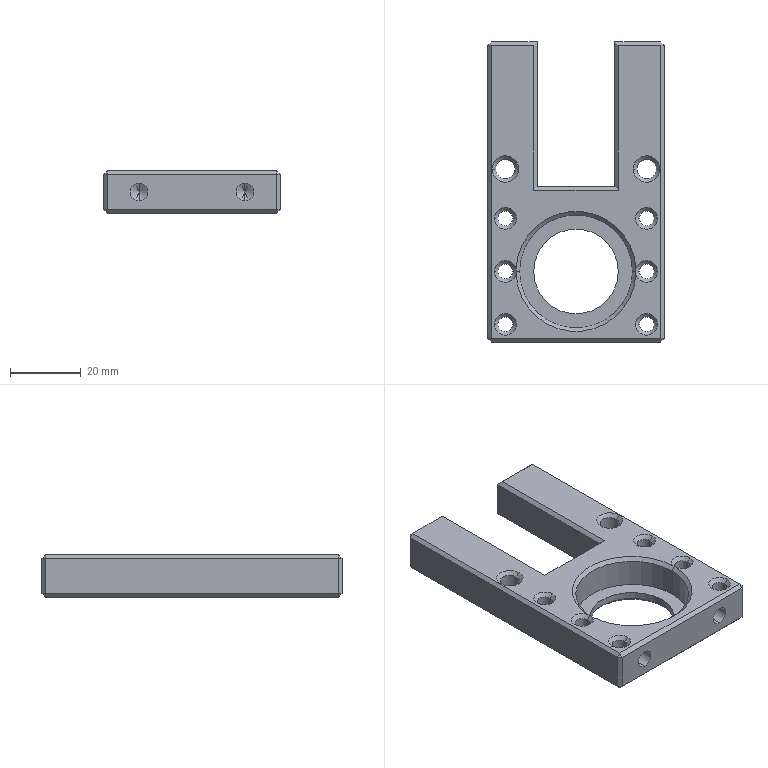Part | STEP file | MT-COMBO-119-S012 | 1 solid | 111 faces | box 50 x 85 x 12 mm | volume 28835 mm3 | cone 44 | plane 39 | cylinder 28 | commonest cylinder face diameters 4.2 x16 5 x4 5.5 x4 24 x2 32 x2